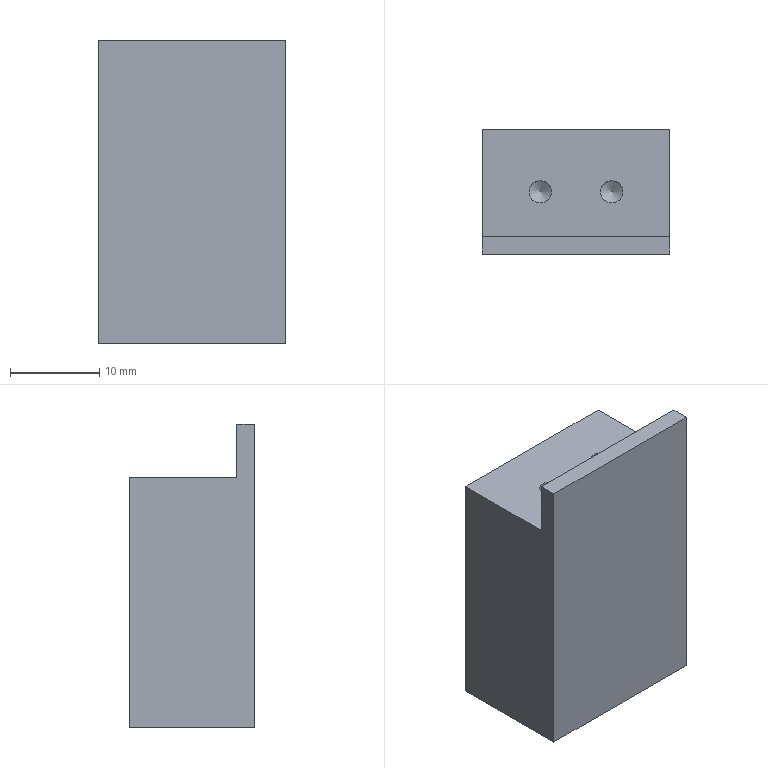Part | NX | 1 solid | 16 faces | box 21 x 14 x 34 mm | volume 8312 mm3 | plane 8 | cone 4 | cylinder 4 | commonest cylinder face diameters 2.5 x4
STEP:
#1=CARTESIAN_POINT('',(5.25,0.,14.));
#2=VERTEX_POINT('',#1);
#3=CARTESIAN_POINT('',(4.,0.,14.));
#4=DIRECTION('',(0.,0.,1.));
#5=DIRECTION('',(1.,0.,0.));
#6=AXIS2_PLACEMENT_3D('',#3,#4,#5);
#7=CIRCLE('',#6,1.25);
#8=EDGE_CURVE('',#2,#2,#7,.T.);
#9=ORIENTED_EDGE('',*,*,#8,.F.);
#10=EDGE_LOOP('',(#9));
#11=FACE_BOUND('',#10,.T.);
#12=CARTESIAN_POINT('',(-2.75,0.,14.));
#13=VERTEX_POINT('',#12);
#14=CARTESIAN_POINT('',(-4.,0.,14.));
#15=DIRECTION('',(0.,0.,1.));
#16=DIRECTION('',(1.,0.,0.));
#17=AXIS2_PLACEMENT_3D('',#14,#15,#16);
#18=CIRCLE('',#17,1.25);
#19=EDGE_CURVE('',#13,#13,#18,.T.);
#20=ORIENTED_EDGE('',*,*,#19,.F.);
#21=EDGE_LOOP('',(#20));
#22=FACE_BOUND('',#21,.T.);
#23=CARTESIAN_POINT('',(10.5,-5.,14.));
#24=VERTEX_POINT('',#23);
#25=CARTESIAN_POINT('',(-10.5,-5.,14.));
#26=VERTEX_POINT('',#25);
#27=CARTESIAN_POINT('',(-10.5,-5.,14.));
#28=DIRECTION('',(-1.,0.,0.));
#29=VECTOR('',#28,1000.);
#30=LINE('',#27,#29);
#31=EDGE_CURVE('',#24,#26,#30,.T.);
#32=ORIENTED_EDGE('',*,*,#31,.F.);
#33=CARTESIAN_POINT('',(10.5,7.,14.));
#34=VERTEX_POINT('',#33);
#35=CARTESIAN_POINT('',(10.5,7.,14.));
#36=DIRECTION('',(0.,-1.,0.));
#37=VECTOR('',#36,1000.);
#38=LINE('',#35,#37);
#39=EDGE_CURVE('',#34,#24,#38,.T.);
#40=ORIENTED_EDGE('',*,*,#39,.F.);
#41=CARTESIAN_POINT('',(-10.5,7.,14.));
#42=VERTEX_POINT('',#41);
#43=CARTESIAN_POINT('',(10.5,7.,14.));
#44=DIRECTION('',(1.,0.,0.));
#45=VECTOR('',#44,1000.);
#46=LINE('',#43,#45);
#47=EDGE_CURVE('',#42,#34,#46,.T.);
#48=ORIENTED_EDGE('',*,*,#47,.F.);
#49=CARTESIAN_POINT('',(-10.5,7.,14.));
#50=DIRECTION('',(0.,-1.,0.));
#51=VECTOR('',#50,1000.);
#52=LINE('',#49,#51);
#53=EDGE_CURVE('',#42,#26,#52,.T.);
#54=ORIENTED_EDGE('',*,*,#53,.T.);
#55=EDGE_LOOP('',(#32,#40,#48,#54));
#56=FACE_BOUND('',#55,.T.);
#57=CARTESIAN_POINT('',(10.5,7.,14.));
#58=DIRECTION('',(0.,0.,-1.));
#59=DIRECTION('',(-1.,0.,0.));
#60=AXIS2_PLACEMENT_3D('',#57,#58,#59);
#61=PLANE('',#60);
#62=ADVANCED_FACE('',(#11,#22,#56),#61,.F.);
#63=CARTESIAN_POINT('',(-10.5,-7.,-14.));
#64=VERTEX_POINT('',#63);
#65=CARTESIAN_POINT('',(-10.5,-7.,20.));
#66=VERTEX_POINT('',#65);
#67=CARTESIAN_POINT('',(-10.5,-7.,14.));
#68=DIRECTION('',(0.,0.,1.));
#69=VECTOR('',#68,1000.);
#70=LINE('',#67,#69);
#71=EDGE_CURVE('',#64,#66,#70,.T.);
#72=ORIENTED_EDGE('',*,*,#71,.T.);
#73=CARTESIAN_POINT('',(-10.5,-5.,20.));
#74=VERTEX_POINT('',#73);
#75=CARTESIAN_POINT('',(-10.5,-7.,20.));
#76=DIRECTION('',(0.,-1.,0.));
#77=VECTOR('',#76,1000.);
#78=LINE('',#75,#77);
#79=EDGE_CURVE('',#74,#66,#78,.T.);
#80=ORIENTED_EDGE('',*,*,#79,.F.);
#81=CARTESIAN_POINT('',(-10.5,-5.,20.));
#82=DIRECTION('',(0.,0.,-1.));
#83=VECTOR('',#82,1000.);
#84=LINE('',#81,#83);
#85=EDGE_CURVE('',#74,#26,#84,.T.);
#86=ORIENTED_EDGE('',*,*,#85,.T.);
#87=ORIENTED_EDGE('',*,*,#53,.F.);
#88=CARTESIAN_POINT('',(-10.5,7.,-14.));
#89=VERTEX_POINT('',#88);
#90=CARTESIAN_POINT('',(-10.5,7.,14.));
#91=DIRECTION('',(0.,0.,1.));
#92=VECTOR('',#91,1000.);
#93=LINE('',#90,#92);
#94=EDGE_CURVE('',#89,#42,#93,.T.);
#95=ORIENTED_EDGE('',*,*,#94,.F.);
#96=CARTESIAN_POINT('',(-10.5,7.,-14.));
#97=DIRECTION('',(0.,-1.,0.));
#98=VECTOR('',#97,1000.);
#99=LINE('',#96,#98);
#100=EDGE_CURVE('',#89,#64,#99,.T.);
#101=ORIENTED_EDGE('',*,*,#100,.T.);
#102=EDGE_LOOP('',(#72,#80,#86,#87,#95,#101));
#103=FACE_BOUND('',#102,.T.);
#104=CARTESIAN_POINT('',(-10.5,7.,14.));
#105=DIRECTION('',(1.,0.,0.));
#106=DIRECTION('',(0.,0.,-1.));
#107=AXIS2_PLACEMENT_3D('',#104,#105,#106);
#108=PLANE('',#107);
#109=ADVANCED_FACE('',(#103),#108,.F.);
#110=CARTESIAN_POINT('',(10.5,-7.,20.));
#111=VERTEX_POINT('',#110);
#112=CARTESIAN_POINT('',(10.5,-7.,-14.));
#113=VERTEX_POINT('',#112);
#114=CARTESIAN_POINT('',(10.5,-7.,14.));
#115=DIRECTION('',(0.,0.,-1.));
#116=VECTOR('',#115,1000.);
#117=LINE('',#114,#116);
#118=EDGE_CURVE('',#111,#113,#117,.T.);
#119=ORIENTED_EDGE('',*,*,#118,.T.);
#120=CARTESIAN_POINT('',(10.5,7.,-14.));
#121=VERTEX_POINT('',#120);
#122=CARTESIAN_POINT('',(10.5,7.,-14.));
#123=DIRECTION('',(0.,-1.,0.));
#124=VECTOR('',#123,1000.);
#125=LINE('',#122,#124);
#126=EDGE_CURVE('',#121,#113,#125,.T.);
#127=ORIENTED_EDGE('',*,*,#126,.F.);
#128=CARTESIAN_POINT('',(10.5,7.,14.));
#129=DIRECTION('',(0.,0.,-1.));
#130=VECTOR('',#129,1000.);
#131=LINE('',#128,#130);
#132=EDGE_CURVE('',#34,#121,#131,.T.);
#133=ORIENTED_EDGE('',*,*,#132,.F.);
#134=ORIENTED_EDGE('',*,*,#39,.T.);
#135=CARTESIAN_POINT('',(10.5,-5.,20.));
#136=VERTEX_POINT('',#135);
#137=CARTESIAN_POINT('',(10.5,-5.,20.));
#138=DIRECTION('',(0.,0.,-1.));
#139=VECTOR('',#138,1000.);
#140=LINE('',#137,#139);
#141=EDGE_CURVE('',#136,#24,#140,.T.);
#142=ORIENTED_EDGE('',*,*,#141,.F.);
#143=CARTESIAN_POINT('',(10.5,-7.,20.));
#144=DIRECTION('',(0.,1.,0.));
#145=VECTOR('',#144,1000.);
#146=LINE('',#143,#145);
#147=EDGE_CURVE('',#111,#136,#146,.T.);
#148=ORIENTED_EDGE('',*,*,#147,.F.);
#149=EDGE_LOOP('',(#119,#127,#133,#134,#142,#148));
#150=FACE_BOUND('',#149,.T.);
#151=CARTESIAN_POINT('',(10.5,7.,14.));
#152=DIRECTION('',(-1.,0.,0.));
#153=DIRECTION('',(0.,0.,1.));
#154=AXIS2_PLACEMENT_3D('',#151,#152,#153);
#155=PLANE('',#154);
#156=ADVANCED_FACE('',(#150),#155,.F.);
#157=CARTESIAN_POINT('',(5.725,3.5,-14.));
#158=VERTEX_POINT('',#157);
#159=CARTESIAN_POINT('',(6.975,3.5,-14.));
#160=DIRECTION('',(0.,0.,-1.));
#161=DIRECTION('',(-1.,0.,0.));
#162=AXIS2_PLACEMENT_3D('',#159,#160,#161);
#163=CIRCLE('',#162,1.25);
#164=EDGE_CURVE('',#158,#158,#163,.T.);
#165=ORIENTED_EDGE('',*,*,#164,.F.);
#166=EDGE_LOOP('',(#165));
#167=FACE_BOUND('',#166,.T.);
#168=CARTESIAN_POINT('',(5.725,-3.5,-14.));
#169=VERTEX_POINT('',#168);
#170=CARTESIAN_POINT('',(6.975,-3.5,-14.));
#171=DIRECTION('',(0.,0.,-1.));
#172=DIRECTION('',(-1.,0.,0.));
#173=AXIS2_PLACEMENT_3D('',#170,#171,#172);
#174=CIRCLE('',#173,1.25);
#175=EDGE_CURVE('',#169,#169,#174,.T.);
#176=ORIENTED_EDGE('',*,*,#175,.F.);
#177=EDGE_LOOP('',(#176));
#178=FACE_BOUND('',#177,.T.);
#179=CARTESIAN_POINT('',(10.5,-7.,-14.));
#180=DIRECTION('',(-1.,0.,0.));
#181=VECTOR('',#180,1000.);
#182=LINE('',#179,#181);
#183=EDGE_CURVE('',#113,#64,#182,.T.);
#184=ORIENTED_EDGE('',*,*,#183,.T.);
#185=ORIENTED_EDGE('',*,*,#100,.F.);
#186=CARTESIAN_POINT('',(10.5,7.,-14.));
#187=DIRECTION('',(-1.,0.,0.));
#188=VECTOR('',#187,1000.);
#189=LINE('',#186,#188);
#190=EDGE_CURVE('',#121,#89,#189,.T.);
#191=ORIENTED_EDGE('',*,*,#190,.F.);
#192=ORIENTED_EDGE('',*,*,#126,.T.);
#193=EDGE_LOOP('',(#184,#185,#191,#192));
#194=FACE_BOUND('',#193,.T.);
#195=CARTESIAN_POINT('',(10.5,7.,-14.));
#196=DIRECTION('',(0.,0.,1.));
#197=DIRECTION('',(1.,0.,0.));
#198=AXIS2_PLACEMENT_3D('',#195,#196,#197);
#199=PLANE('',#198);
#200=ADVANCED_FACE('',(#167,#178,#194),#199,.F.);
#201=ORIENTED_EDGE('',*,*,#94,.T.);
#202=ORIENTED_EDGE('',*,*,#47,.T.);
#203=ORIENTED_EDGE('',*,*,#132,.T.);
#204=ORIENTED_EDGE('',*,*,#190,.T.);
#205=EDGE_LOOP('',(#201,#202,#203,#204));
#206=FACE_BOUND('',#205,.T.);
#207=CARTESIAN_POINT('',(0.,7.,0.));
#208=DIRECTION('',(0.,1.,0.));
#209=DIRECTION('',(0.,0.,1.));
#210=AXIS2_PLACEMENT_3D('',#207,#208,#209);
#211=PLANE('',#210);
#212=ADVANCED_FACE('',(#206),#211,.T.);
#213=ORIENTED_EDGE('',*,*,#71,.F.);
#214=ORIENTED_EDGE('',*,*,#183,.F.);
#215=ORIENTED_EDGE('',*,*,#118,.F.);
#216=CARTESIAN_POINT('',(-10.5,-7.,20.));
#217=DIRECTION('',(1.,0.,0.));
#218=VECTOR('',#217,1000.);
#219=LINE('',#216,#218);
#220=EDGE_CURVE('',#66,#111,#219,.T.);
#221=ORIENTED_EDGE('',*,*,#220,.F.);
#222=EDGE_LOOP('',(#213,#214,#215,#221));
#223=FACE_BOUND('',#222,.T.);
#224=CARTESIAN_POINT('',(0.,-7.,0.));
#225=DIRECTION('',(0.,1.,0.));
#226=DIRECTION('',(0.,0.,1.));
#227=AXIS2_PLACEMENT_3D('',#224,#225,#226);
#228=PLANE('',#227);
#229=ADVANCED_FACE('',(#223),#228,.F.);
#230=CARTESIAN_POINT('',(6.975,-3.5,-4.749));
#231=VERTEX_POINT('',#230);
#232=VERTEX_LOOP('',#231);
#233=FACE_BOUND('',#232,.T.);
#234=CARTESIAN_POINT('',(5.725,-3.5,-5.5));
#235=VERTEX_POINT('',#234);
#236=CARTESIAN_POINT('',(6.975,-3.5,-5.5));
#237=DIRECTION('',(0.,0.,-1.));
#238=DIRECTION('',(-1.,0.,0.));
#239=AXIS2_PLACEMENT_3D('',#236,#237,#238);
#240=CIRCLE('',#239,1.25);
#241=EDGE_CURVE('',#235,#235,#240,.T.);
#242=ORIENTED_EDGE('',*,*,#241,.T.);
#243=EDGE_LOOP('',(#242));
#244=FACE_BOUND('',#243,.T.);
#245=CARTESIAN_POINT('',(6.975,-3.5,-5.5));
#246=DIRECTION('',(0.,0.,-1.));
#247=DIRECTION('',(-1.,0.,0.));
#248=AXIS2_PLACEMENT_3D('',#245,#246,#247);
#249=CONICAL_SURFACE('',#248,1.25,1.03);
#250=ADVANCED_FACE('',(#233,#244),#249,.F.);
#251=ORIENTED_EDGE('',*,*,#241,.F.);
#252=EDGE_LOOP('',(#251));
#253=FACE_BOUND('',#252,.T.);
#254=ORIENTED_EDGE('',*,*,#175,.T.);
#255=EDGE_LOOP('',(#254));
#256=FACE_BOUND('',#255,.T.);
#257=CARTESIAN_POINT('',(6.975,-3.5,-14.));
#258=DIRECTION('',(0.,0.,-1.));
#259=DIRECTION('',(-1.,0.,0.));
#260=AXIS2_PLACEMENT_3D('',#257,#258,#259);
#261=CYLINDRICAL_SURFACE('',#260,1.25);
#262=ADVANCED_FACE('',(#253,#256),#261,.F.);
#263=CARTESIAN_POINT('',(6.975,3.5,-4.749));
#264=VERTEX_POINT('',#263);
#265=VERTEX_LOOP('',#264);
#266=FACE_BOUND('',#265,.T.);
#267=CARTESIAN_POINT('',(5.725,3.5,-5.5));
#268=VERTEX_POINT('',#267);
#269=CARTESIAN_POINT('',(6.975,3.5,-5.5));
#270=DIRECTION('',(0.,0.,-1.));
#271=DIRECTION('',(-1.,0.,0.));
#272=AXIS2_PLACEMENT_3D('',#269,#270,#271);
#273=CIRCLE('',#272,1.25);
#274=EDGE_CURVE('',#268,#268,#273,.T.);
#275=ORIENTED_EDGE('',*,*,#274,.T.);
#276=EDGE_LOOP('',(#275));
#277=FACE_BOUND('',#276,.T.);
#278=CARTESIAN_POINT('',(6.975,3.5,-5.5));
#279=DIRECTION('',(0.,0.,-1.));
#280=DIRECTION('',(-1.,0.,0.));
#281=AXIS2_PLACEMENT_3D('',#278,#279,#280);
#282=CONICAL_SURFACE('',#281,1.25,1.03);
#283=ADVANCED_FACE('',(#266,#277),#282,.F.);
#284=ORIENTED_EDGE('',*,*,#274,.F.);
#285=EDGE_LOOP('',(#284));
#286=FACE_BOUND('',#285,.T.);
#287=ORIENTED_EDGE('',*,*,#164,.T.);
#288=EDGE_LOOP('',(#287));
#289=FACE_BOUND('',#288,.T.);
#290=CARTESIAN_POINT('',(6.975,3.5,-14.));
#291=DIRECTION('',(0.,0.,-1.));
#292=DIRECTION('',(-1.,0.,0.));
#293=AXIS2_PLACEMENT_3D('',#290,#291,#292);
#294=CYLINDRICAL_SURFACE('',#293,1.25);
#295=ADVANCED_FACE('',(#286,#289),#294,.F.);
#296=CARTESIAN_POINT('',(4.,0.,4.749));
#297=VERTEX_POINT('',#296);
#298=VERTEX_LOOP('',#297);
#299=FACE_BOUND('',#298,.T.);
#300=CARTESIAN_POINT('',(5.25,0.,5.5));
#301=VERTEX_POINT('',#300);
#302=CARTESIAN_POINT('',(4.,0.,5.5));
#303=DIRECTION('',(0.,0.,1.));
#304=DIRECTION('',(1.,0.,0.));
#305=AXIS2_PLACEMENT_3D('',#302,#303,#304);
#306=CIRCLE('',#305,1.25);
#307=EDGE_CURVE('',#301,#301,#306,.T.);
#308=ORIENTED_EDGE('',*,*,#307,.T.);
#309=EDGE_LOOP('',(#308));
#310=FACE_BOUND('',#309,.T.);
#311=CARTESIAN_POINT('',(4.,0.,5.5));
#312=DIRECTION('',(0.,0.,1.));
#313=DIRECTION('',(1.,0.,0.));
#314=AXIS2_PLACEMENT_3D('',#311,#312,#313);
#315=CONICAL_SURFACE('',#314,1.25,1.03);
#316=ADVANCED_FACE('',(#299,#310),#315,.F.);
#317=ORIENTED_EDGE('',*,*,#307,.F.);
#318=EDGE_LOOP('',(#317));
#319=FACE_BOUND('',#318,.T.);
#320=ORIENTED_EDGE('',*,*,#8,.T.);
#321=EDGE_LOOP('',(#320));
#322=FACE_BOUND('',#321,.T.);
#323=CARTESIAN_POINT('',(4.,0.,14.));
#324=DIRECTION('',(0.,0.,1.));
#325=DIRECTION('',(1.,0.,0.));
#326=AXIS2_PLACEMENT_3D('',#323,#324,#325);
#327=CYLINDRICAL_SURFACE('',#326,1.25);
#328=ADVANCED_FACE('',(#319,#322),#327,.F.);
#329=CARTESIAN_POINT('',(-4.,0.,4.749));
#330=VERTEX_POINT('',#329);
#331=VERTEX_LOOP('',#330);
#332=FACE_BOUND('',#331,.T.);
#333=CARTESIAN_POINT('',(-2.75,0.,5.5));
#334=VERTEX_POINT('',#333);
#335=CARTESIAN_POINT('',(-4.,0.,5.5));
#336=DIRECTION('',(0.,0.,1.));
#337=DIRECTION('',(1.,0.,0.));
#338=AXIS2_PLACEMENT_3D('',#335,#336,#337);
#339=CIRCLE('',#338,1.25);
#340=EDGE_CURVE('',#334,#334,#339,.T.);
#341=ORIENTED_EDGE('',*,*,#340,.T.);
#342=EDGE_LOOP('',(#341));
#343=FACE_BOUND('',#342,.T.);
#344=CARTESIAN_POINT('',(-4.,0.,5.5));
#345=DIRECTION('',(0.,0.,1.));
#346=DIRECTION('',(1.,0.,0.));
#347=AXIS2_PLACEMENT_3D('',#344,#345,#346);
#348=CONICAL_SURFACE('',#347,1.25,1.03);
#349=ADVANCED_FACE('',(#332,#343),#348,.F.);
#350=ORIENTED_EDGE('',*,*,#340,.F.);
#351=EDGE_LOOP('',(#350));
#352=FACE_BOUND('',#351,.T.);
#353=ORIENTED_EDGE('',*,*,#19,.T.);
#354=EDGE_LOOP('',(#353));
#355=FACE_BOUND('',#354,.T.);
#356=CARTESIAN_POINT('',(-4.,0.,14.));
#357=DIRECTION('',(0.,0.,1.));
#358=DIRECTION('',(1.,0.,0.));
#359=AXIS2_PLACEMENT_3D('',#356,#357,#358);
#360=CYLINDRICAL_SURFACE('',#359,1.25);
#361=ADVANCED_FACE('',(#352,#355),#360,.F.);
#362=ORIENTED_EDGE('',*,*,#31,.T.);
#363=ORIENTED_EDGE('',*,*,#85,.F.);
#364=CARTESIAN_POINT('',(-10.5,-5.,20.));
#365=DIRECTION('',(-1.,0.,0.));
#366=VECTOR('',#365,1000.);
#367=LINE('',#364,#366);
#368=EDGE_CURVE('',#136,#74,#367,.T.);
#369=ORIENTED_EDGE('',*,*,#368,.F.);
#370=ORIENTED_EDGE('',*,*,#141,.T.);
#371=EDGE_LOOP('',(#362,#363,#369,#370));
#372=FACE_BOUND('',#371,.T.);
#373=CARTESIAN_POINT('',(-10.5,-5.,20.));
#374=DIRECTION('',(0.,-1.,0.));
#375=DIRECTION('',(0.,0.,-1.));
#376=AXIS2_PLACEMENT_3D('',#373,#374,#375);
#377=PLANE('',#376);
#378=ADVANCED_FACE('',(#372),#377,.F.);
#379=ORIENTED_EDGE('',*,*,#79,.T.);
#380=ORIENTED_EDGE('',*,*,#220,.T.);
#381=ORIENTED_EDGE('',*,*,#147,.T.);
#382=ORIENTED_EDGE('',*,*,#368,.T.);
#383=EDGE_LOOP('',(#379,#380,#381,#382));
#384=FACE_BOUND('',#383,.T.);
#385=CARTESIAN_POINT('',(0.,0.,20.));
#386=DIRECTION('',(0.,0.,-1.));
#387=DIRECTION('',(-1.,0.,0.));
#388=AXIS2_PLACEMENT_3D('',#385,#386,#387);
#389=PLANE('',#388);
#390=ADVANCED_FACE('',(#384),#389,.F.);
#391=CLOSED_SHELL('',(#62,#109,#156,#200,#212,#229,#250,#262,#283,#295,#316,#328,#349,#361,#378,#390));
#392=MANIFOLD_SOLID_BREP('',#391);
#393=(LENGTH_UNIT()NAMED_UNIT(*)SI_UNIT(.MILLI.,.METRE.));
#394=UNCERTAINTY_MEASURE_WITH_UNIT(LENGTH_MEASURE(0.00001),#393,'','');
#395=(NAMED_UNIT(*)PLANE_ANGLE_UNIT()SI_UNIT($,.RADIAN.));
#396=(NAMED_UNIT(*)SI_UNIT($,.STERADIAN.)SOLID_ANGLE_UNIT());
#397=(GEOMETRIC_REPRESENTATION_CONTEXT(3)GLOBAL_UNCERTAINTY_ASSIGNED_CONTEXT((#394))GLOBAL_UNIT_ASSIGNED_CONTEXT((#393,#395,#396))REPRESENTATION_CONTEXT('',''));
#398=ADVANCED_BREP_SHAPE_REPRESENTATION('',(#392),#397);